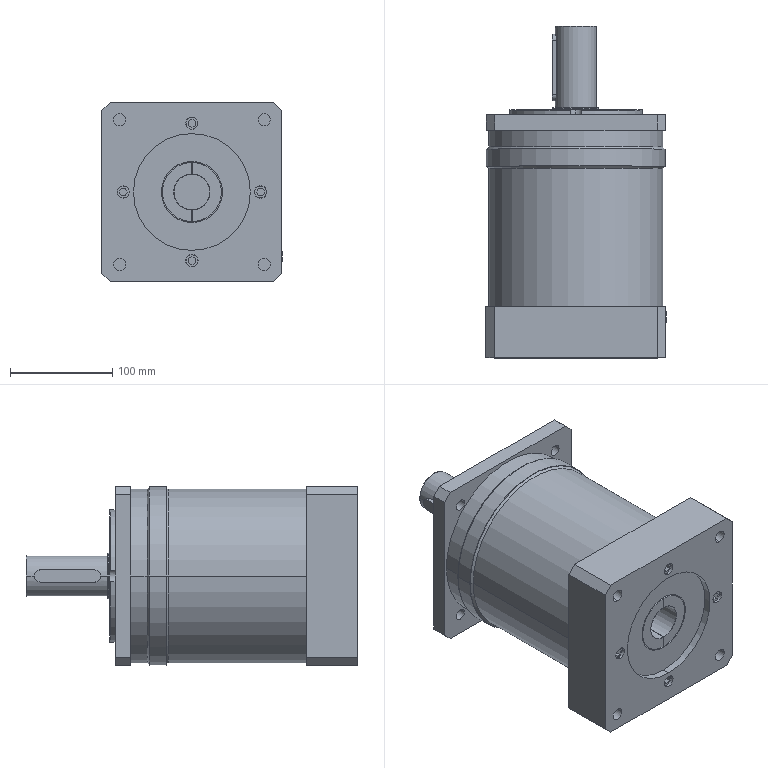Part | SolidWorks | features ICE 15, CirPattern 7, Fillet 5, Chamfer 4, 3DProfileFeature 1, CombineBodies 1, HoleWzd 1, RefAxis 1, Revolution 1 | 1 solid | 289 faces | box 176.2 x 324.5 x 176 mm | volume 5934873 mm3 | plane 150 | cylinder 105 | torus 26 | cone 8 | commonest cylinder face diameters 12 x28 11.8 x16 98 x12 114 x12 11 x8 57.86 x5